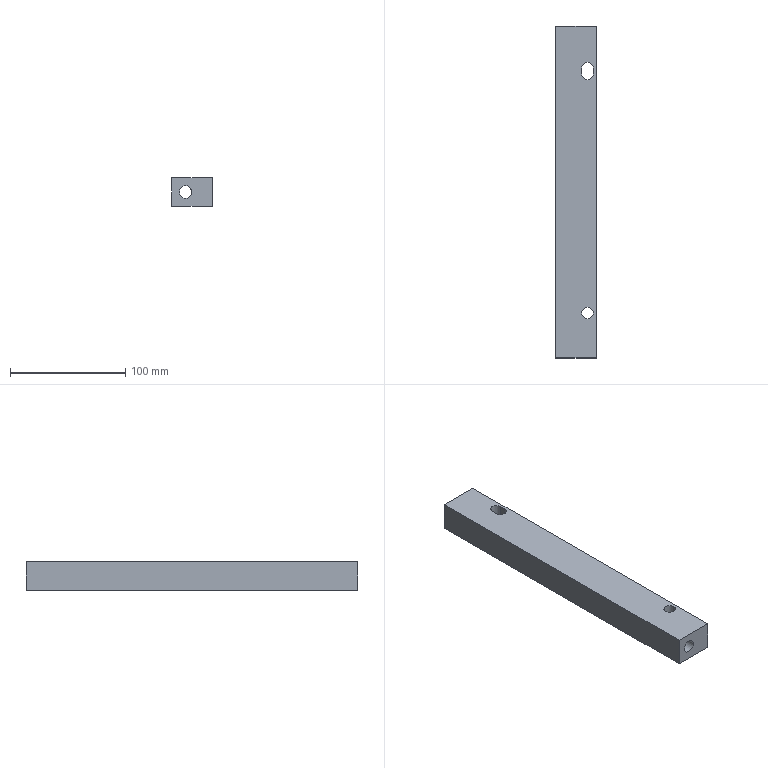Part | NX | features solid 2 | 1 solid | 19 faces | box 35 x 288 x 25 mm | volume 207259 mm3 | cylinder 11 | plane 8 | commonest cylinder face diameters 11 x8 10 x3
STEP:
#1=CARTESIAN_POINT('',(42.5,-250.,340.));
#2=VERTEX_POINT('',#1);
#3=CARTESIAN_POINT('',(47.5,-250.,340.));
#4=DIRECTION('',(0.,0.,-1.));
#5=DIRECTION('',(-1.,0.,0.));
#6=AXIS2_PLACEMENT_3D('',#3,#4,#5);
#7=CIRCLE('',#6,5.);
#8=EDGE_CURVE('',#2,#2,#7,.T.);
#9=ORIENTED_EDGE('',*,*,#8,.T.);
#10=EDGE_LOOP('',(#9));
#11=FACE_BOUND('',#10,.T.);
#12=CARTESIAN_POINT('',(52.5,-37.5,340.));
#13=VERTEX_POINT('',#12);
#14=CARTESIAN_POINT('',(52.5,-42.5,340.));
#15=VERTEX_POINT('',#14);
#16=CARTESIAN_POINT('',(52.5,-145.,340.));
#17=DIRECTION('',(0.,-1.,0.));
#18=VECTOR('',#17,1000.);
#19=LINE('',#16,#18);
#20=EDGE_CURVE('',#13,#15,#19,.T.);
#21=ORIENTED_EDGE('',*,*,#20,.T.);
#22=CARTESIAN_POINT('',(42.5,-42.5,340.));
#23=VERTEX_POINT('',#22);
#24=CARTESIAN_POINT('',(47.5,-42.5,340.));
#25=DIRECTION('',(0.,0.,-1.));
#26=DIRECTION('',(-1.,0.,0.));
#27=AXIS2_PLACEMENT_3D('',#24,#25,#26);
#28=CIRCLE('',#27,5.);
#29=EDGE_CURVE('',#15,#23,#28,.T.);
#30=ORIENTED_EDGE('',*,*,#29,.T.);
#31=CARTESIAN_POINT('',(42.5,-37.5,340.));
#32=VERTEX_POINT('',#31);
#33=CARTESIAN_POINT('',(42.5,-145.,340.));
#34=DIRECTION('',(0.,1.,0.));
#35=VECTOR('',#34,1000.);
#36=LINE('',#33,#35);
#37=EDGE_CURVE('',#23,#32,#36,.T.);
#38=ORIENTED_EDGE('',*,*,#37,.T.);
#39=CARTESIAN_POINT('',(47.5,-37.5,340.));
#40=DIRECTION('',(0.,0.,-1.));
#41=DIRECTION('',(-1.,0.,0.));
#42=AXIS2_PLACEMENT_3D('',#39,#40,#41);
#43=CIRCLE('',#42,5.);
#44=EDGE_CURVE('',#32,#13,#43,.T.);
#45=ORIENTED_EDGE('',*,*,#44,.T.);
#46=EDGE_LOOP('',(#21,#30,#38,#45));
#47=FACE_BOUND('',#46,.T.);
#48=CARTESIAN_POINT('',(20.,-289.,340.));
#49=VERTEX_POINT('',#48);
#50=CARTESIAN_POINT('',(55.,-289.,340.));
#51=VERTEX_POINT('',#50);
#52=CARTESIAN_POINT('',(37.5,-289.,340.));
#53=DIRECTION('',(1.,0.,0.));
#54=VECTOR('',#53,1000.);
#55=LINE('',#52,#54);
#56=EDGE_CURVE('',#49,#51,#55,.T.);
#57=ORIENTED_EDGE('',*,*,#56,.T.);
#58=CARTESIAN_POINT('',(55.,-1.,340.));
#59=VERTEX_POINT('',#58);
#60=CARTESIAN_POINT('',(55.,-145.,340.));
#61=DIRECTION('',(0.,1.,0.));
#62=VECTOR('',#61,1000.);
#63=LINE('',#60,#62);
#64=EDGE_CURVE('',#51,#59,#63,.T.);
#65=ORIENTED_EDGE('',*,*,#64,.T.);
#66=CARTESIAN_POINT('',(20.,-1.,340.));
#67=VERTEX_POINT('',#66);
#68=CARTESIAN_POINT('',(37.5,-1.,340.));
#69=DIRECTION('',(-1.,0.,0.));
#70=VECTOR('',#69,1000.);
#71=LINE('',#68,#70);
#72=EDGE_CURVE('',#59,#67,#71,.T.);
#73=ORIENTED_EDGE('',*,*,#72,.T.);
#74=CARTESIAN_POINT('',(20.,-145.,340.));
#75=DIRECTION('',(0.,-1.,0.));
#76=VECTOR('',#75,1000.);
#77=LINE('',#74,#76);
#78=EDGE_CURVE('',#67,#49,#77,.T.);
#79=ORIENTED_EDGE('',*,*,#78,.T.);
#80=EDGE_LOOP('',(#57,#65,#73,#79));
#81=FACE_BOUND('',#80,.T.);
#82=CARTESIAN_POINT('',(37.5,-145.,340.));
#83=DIRECTION('',(0.,0.,1.));
#84=DIRECTION('',(-1.,0.,0.));
#85=AXIS2_PLACEMENT_3D('',#82,#83,#84);
#86=PLANE('',#85);
#87=ADVANCED_FACE('',(#11,#47,#81),#86,.T.);
#88=CARTESIAN_POINT('',(32.,-289.,322.));
#89=VERTEX_POINT('',#88);
#90=CARTESIAN_POINT('',(32.,-289.,327.5));
#91=DIRECTION('',(0.,1.,0.));
#92=DIRECTION('',(0.,0.,-1.));
#93=AXIS2_PLACEMENT_3D('',#90,#91,#92);
#94=CIRCLE('',#93,5.5);
#95=EDGE_CURVE('',#89,#89,#94,.T.);
#96=ORIENTED_EDGE('',*,*,#95,.T.);
#97=EDGE_LOOP('',(#96));
#98=FACE_BOUND('',#97,.T.);
#99=CARTESIAN_POINT('',(20.,-289.,315.));
#100=VERTEX_POINT('',#99);
#101=CARTESIAN_POINT('',(20.,-289.,315.));
#102=DIRECTION('',(0.,0.,1.));
#103=VECTOR('',#102,1000.);
#104=LINE('',#101,#103);
#105=EDGE_CURVE('',#100,#49,#104,.T.);
#106=ORIENTED_EDGE('',*,*,#105,.F.);
#107=CARTESIAN_POINT('',(55.,-289.,315.));
#108=VERTEX_POINT('',#107);
#109=CARTESIAN_POINT('',(37.5,-289.,315.));
#110=DIRECTION('',(-1.,0.,0.));
#111=VECTOR('',#110,1000.);
#112=LINE('',#109,#111);
#113=EDGE_CURVE('',#108,#100,#112,.T.);
#114=ORIENTED_EDGE('',*,*,#113,.F.);
#115=CARTESIAN_POINT('',(55.,-289.,315.));
#116=DIRECTION('',(0.,0.,1.));
#117=VECTOR('',#116,1000.);
#118=LINE('',#115,#117);
#119=EDGE_CURVE('',#108,#51,#118,.T.);
#120=ORIENTED_EDGE('',*,*,#119,.T.);
#121=ORIENTED_EDGE('',*,*,#56,.F.);
#122=EDGE_LOOP('',(#106,#114,#120,#121));
#123=FACE_BOUND('',#122,.T.);
#124=CARTESIAN_POINT('',(37.5,-289.,315.));
#125=DIRECTION('',(0.,-1.,0.));
#126=DIRECTION('',(0.,0.,-1.));
#127=AXIS2_PLACEMENT_3D('',#124,#125,#126);
#128=PLANE('',#127);
#129=ADVANCED_FACE('',(#98,#123),#128,.T.);
#130=CARTESIAN_POINT('',(55.,-271.,322.));
#131=VERTEX_POINT('',#130);
#132=CARTESIAN_POINT('',(55.,-271.,327.5));
#133=DIRECTION('',(1.,0.,0.));
#134=DIRECTION('',(0.,0.,-1.));
#135=AXIS2_PLACEMENT_3D('',#132,#133,#134);
#136=CIRCLE('',#135,5.5);
#137=EDGE_CURVE('',#131,#131,#136,.T.);
#138=ORIENTED_EDGE('',*,*,#137,.F.);
#139=EDGE_LOOP('',(#138));
#140=FACE_BOUND('',#139,.T.);
#141=CARTESIAN_POINT('',(55.,-229.,322.));
#142=VERTEX_POINT('',#141);
#143=CARTESIAN_POINT('',(55.,-229.,327.5));
#144=DIRECTION('',(1.,0.,0.));
#145=DIRECTION('',(0.,0.,-1.));
#146=AXIS2_PLACEMENT_3D('',#143,#144,#145);
#147=CIRCLE('',#146,5.5);
#148=EDGE_CURVE('',#142,#142,#147,.T.);
#149=ORIENTED_EDGE('',*,*,#148,.F.);
#150=EDGE_LOOP('',(#149));
#151=FACE_BOUND('',#150,.T.);
#152=CARTESIAN_POINT('',(55.,-187.,322.));
#153=VERTEX_POINT('',#152);
#154=CARTESIAN_POINT('',(55.,-187.,327.5));
#155=DIRECTION('',(1.,0.,0.));
#156=DIRECTION('',(0.,0.,-1.));
#157=AXIS2_PLACEMENT_3D('',#154,#155,#156);
#158=CIRCLE('',#157,5.5);
#159=EDGE_CURVE('',#153,#153,#158,.T.);
#160=ORIENTED_EDGE('',*,*,#159,.F.);
#161=EDGE_LOOP('',(#160));
#162=FACE_BOUND('',#161,.T.);
#163=CARTESIAN_POINT('',(55.,-145.,322.));
#164=VERTEX_POINT('',#163);
#165=CARTESIAN_POINT('',(55.,-145.,327.5));
#166=DIRECTION('',(1.,0.,0.));
#167=DIRECTION('',(0.,0.,-1.));
#168=AXIS2_PLACEMENT_3D('',#165,#166,#167);
#169=CIRCLE('',#168,5.5);
#170=EDGE_CURVE('',#164,#164,#169,.T.);
#171=ORIENTED_EDGE('',*,*,#170,.F.);
#172=EDGE_LOOP('',(#171));
#173=FACE_BOUND('',#172,.T.);
#174=CARTESIAN_POINT('',(55.,-103.,322.));
#175=VERTEX_POINT('',#174);
#176=CARTESIAN_POINT('',(55.,-103.,327.5));
#177=DIRECTION('',(1.,0.,0.));
#178=DIRECTION('',(0.,0.,-1.));
#179=AXIS2_PLACEMENT_3D('',#176,#177,#178);
#180=CIRCLE('',#179,5.5);
#181=EDGE_CURVE('',#175,#175,#180,.T.);
#182=ORIENTED_EDGE('',*,*,#181,.F.);
#183=EDGE_LOOP('',(#182));
#184=FACE_BOUND('',#183,.T.);
#185=CARTESIAN_POINT('',(55.,-61.,322.));
#186=VERTEX_POINT('',#185);
#187=CARTESIAN_POINT('',(55.,-61.,327.5));
#188=DIRECTION('',(1.,0.,0.));
#189=DIRECTION('',(0.,0.,-1.));
#190=AXIS2_PLACEMENT_3D('',#187,#188,#189);
#191=CIRCLE('',#190,5.5);
#192=EDGE_CURVE('',#186,#186,#191,.T.);
#193=ORIENTED_EDGE('',*,*,#192,.F.);
#194=EDGE_LOOP('',(#193));
#195=FACE_BOUND('',#194,.T.);
#196=CARTESIAN_POINT('',(55.,-19.,322.));
#197=VERTEX_POINT('',#196);
#198=CARTESIAN_POINT('',(55.,-19.,327.5));
#199=DIRECTION('',(1.,0.,0.));
#200=DIRECTION('',(0.,0.,-1.));
#201=AXIS2_PLACEMENT_3D('',#198,#199,#200);
#202=CIRCLE('',#201,5.5);
#203=EDGE_CURVE('',#197,#197,#202,.T.);
#204=ORIENTED_EDGE('',*,*,#203,.F.);
#205=EDGE_LOOP('',(#204));
#206=FACE_BOUND('',#205,.T.);
#207=ORIENTED_EDGE('',*,*,#119,.F.);
#208=CARTESIAN_POINT('',(55.,-1.,315.));
#209=VERTEX_POINT('',#208);
#210=CARTESIAN_POINT('',(55.,-145.,315.));
#211=DIRECTION('',(0.,-1.,0.));
#212=VECTOR('',#211,1000.);
#213=LINE('',#210,#212);
#214=EDGE_CURVE('',#209,#108,#213,.T.);
#215=ORIENTED_EDGE('',*,*,#214,.F.);
#216=CARTESIAN_POINT('',(55.,-1.,315.));
#217=DIRECTION('',(0.,0.,1.));
#218=VECTOR('',#217,1000.);
#219=LINE('',#216,#218);
#220=EDGE_CURVE('',#209,#59,#219,.T.);
#221=ORIENTED_EDGE('',*,*,#220,.T.);
#222=ORIENTED_EDGE('',*,*,#64,.F.);
#223=EDGE_LOOP('',(#207,#215,#221,#222));
#224=FACE_BOUND('',#223,.T.);
#225=CARTESIAN_POINT('',(55.,-145.,315.));
#226=DIRECTION('',(1.,0.,0.));
#227=DIRECTION('',(0.,0.,1.));
#228=AXIS2_PLACEMENT_3D('',#225,#226,#227);
#229=PLANE('',#228);
#230=ADVANCED_FACE('',(#140,#151,#162,#173,#184,#195,#206,#224),#229,.T.);
#231=CARTESIAN_POINT('',(32.,-1.,322.));
#232=VERTEX_POINT('',#231);
#233=CARTESIAN_POINT('',(32.,-1.,327.5));
#234=DIRECTION('',(0.,1.,0.));
#235=DIRECTION('',(0.,0.,-1.));
#236=AXIS2_PLACEMENT_3D('',#233,#234,#235);
#237=CIRCLE('',#236,5.5);
#238=EDGE_CURVE('',#232,#232,#237,.T.);
#239=ORIENTED_EDGE('',*,*,#238,.F.);
#240=EDGE_LOOP('',(#239));
#241=FACE_BOUND('',#240,.T.);
#242=ORIENTED_EDGE('',*,*,#220,.F.);
#243=CARTESIAN_POINT('',(20.,-1.,315.));
#244=VERTEX_POINT('',#243);
#245=CARTESIAN_POINT('',(37.5,-1.,315.));
#246=DIRECTION('',(1.,0.,0.));
#247=VECTOR('',#246,1000.);
#248=LINE('',#245,#247);
#249=EDGE_CURVE('',#244,#209,#248,.T.);
#250=ORIENTED_EDGE('',*,*,#249,.F.);
#251=CARTESIAN_POINT('',(20.,-1.,315.));
#252=DIRECTION('',(0.,0.,1.));
#253=VECTOR('',#252,1000.);
#254=LINE('',#251,#253);
#255=EDGE_CURVE('',#244,#67,#254,.T.);
#256=ORIENTED_EDGE('',*,*,#255,.T.);
#257=ORIENTED_EDGE('',*,*,#72,.F.);
#258=EDGE_LOOP('',(#242,#250,#256,#257));
#259=FACE_BOUND('',#258,.T.);
#260=CARTESIAN_POINT('',(37.5,-1.,315.));
#261=DIRECTION('',(0.,1.,0.));
#262=DIRECTION('',(0.,0.,1.));
#263=AXIS2_PLACEMENT_3D('',#260,#261,#262);
#264=PLANE('',#263);
#265=ADVANCED_FACE('',(#241,#259),#264,.T.);
#266=CARTESIAN_POINT('',(42.5,-250.,315.));
#267=VERTEX_POINT('',#266);
#268=CARTESIAN_POINT('',(47.5,-250.,315.));
#269=DIRECTION('',(0.,0.,-1.));
#270=DIRECTION('',(-1.,0.,0.));
#271=AXIS2_PLACEMENT_3D('',#268,#269,#270);
#272=CIRCLE('',#271,5.);
#273=EDGE_CURVE('',#267,#267,#272,.T.);
#274=ORIENTED_EDGE('',*,*,#273,.F.);
#275=EDGE_LOOP('',(#274));
#276=FACE_BOUND('',#275,.T.);
#277=CARTESIAN_POINT('',(52.5,-37.5,315.));
#278=VERTEX_POINT('',#277);
#279=CARTESIAN_POINT('',(52.5,-42.5,315.));
#280=VERTEX_POINT('',#279);
#281=CARTESIAN_POINT('',(52.5,-40.,315.));
#282=DIRECTION('',(0.,-1.,0.));
#283=VECTOR('',#282,1000.);
#284=LINE('',#281,#283);
#285=EDGE_CURVE('',#278,#280,#284,.T.);
#286=ORIENTED_EDGE('',*,*,#285,.F.);
#287=CARTESIAN_POINT('',(42.5,-37.5,315.));
#288=VERTEX_POINT('',#287);
#289=CARTESIAN_POINT('',(47.5,-37.5,315.));
#290=DIRECTION('',(0.,0.,1.));
#291=DIRECTION('',(1.,0.,0.));
#292=AXIS2_PLACEMENT_3D('',#289,#290,#291);
#293=CIRCLE('',#292,5.);
#294=EDGE_CURVE('',#278,#288,#293,.T.);
#295=ORIENTED_EDGE('',*,*,#294,.T.);
#296=CARTESIAN_POINT('',(42.5,-42.5,315.));
#297=VERTEX_POINT('',#296);
#298=CARTESIAN_POINT('',(42.5,-40.,315.));
#299=DIRECTION('',(0.,-1.,0.));
#300=VECTOR('',#299,1000.);
#301=LINE('',#298,#300);
#302=EDGE_CURVE('',#288,#297,#301,.T.);
#303=ORIENTED_EDGE('',*,*,#302,.T.);
#304=CARTESIAN_POINT('',(47.5,-42.5,315.));
#305=DIRECTION('',(0.,0.,1.));
#306=DIRECTION('',(1.,0.,0.));
#307=AXIS2_PLACEMENT_3D('',#304,#305,#306);
#308=CIRCLE('',#307,5.);
#309=EDGE_CURVE('',#297,#280,#308,.T.);
#310=ORIENTED_EDGE('',*,*,#309,.T.);
#311=EDGE_LOOP('',(#286,#295,#303,#310));
#312=FACE_BOUND('',#311,.T.);
#313=CARTESIAN_POINT('',(20.,-145.,315.));
#314=DIRECTION('',(0.,1.,0.));
#315=VECTOR('',#314,1000.);
#316=LINE('',#313,#315);
#317=EDGE_CURVE('',#100,#244,#316,.T.);
#318=ORIENTED_EDGE('',*,*,#317,.T.);
#319=ORIENTED_EDGE('',*,*,#249,.T.);
#320=ORIENTED_EDGE('',*,*,#214,.T.);
#321=ORIENTED_EDGE('',*,*,#113,.T.);
#322=EDGE_LOOP('',(#318,#319,#320,#321));
#323=FACE_BOUND('',#322,.T.);
#324=CARTESIAN_POINT('',(37.5,-145.,315.));
#325=DIRECTION('',(0.,0.,-1.));
#326=DIRECTION('',(1.,0.,0.));
#327=AXIS2_PLACEMENT_3D('',#324,#325,#326);
#328=PLANE('',#327);
#329=ADVANCED_FACE('',(#276,#312,#323),#328,.T.);
#330=ORIENTED_EDGE('',*,*,#317,.F.);
#331=ORIENTED_EDGE('',*,*,#105,.T.);
#332=ORIENTED_EDGE('',*,*,#78,.F.);
#333=ORIENTED_EDGE('',*,*,#255,.F.);
#334=EDGE_LOOP('',(#330,#331,#332,#333));
#335=FACE_BOUND('',#334,.T.);
#336=CARTESIAN_POINT('',(20.,-145.,315.));
#337=DIRECTION('',(-1.,0.,0.));
#338=DIRECTION('',(0.,0.,-1.));
#339=AXIS2_PLACEMENT_3D('',#336,#337,#338);
#340=PLANE('',#339);
#341=ADVANCED_FACE('',(#335),#340,.T.);
#342=CARTESIAN_POINT('',(32.,-271.,333.));
#343=VERTEX_POINT('',#342);
#344=CARTESIAN_POINT('',(32.,-271.,322.));
#345=VERTEX_POINT('',#344);
#346=CARTESIAN_POINT('',(32.,-271.,327.5));
#347=DIRECTION('',(-0.7071,0.7071,0.));
#348=DIRECTION('',(-0.7071,-0.7071,0.));
#349=AXIS2_PLACEMENT_3D('',#346,#347,#348);
#350=ELLIPSE('',#349,7.778,5.5);
#351=EDGE_CURVE('',#343,#345,#350,.T.);
#352=ORIENTED_EDGE('',*,*,#351,.F.);
#353=CARTESIAN_POINT('',(32.,-271.,327.5));
#354=DIRECTION('',(0.7071,0.7071,0.));
#355=DIRECTION('',(0.7071,-0.7071,0.));
#356=AXIS2_PLACEMENT_3D('',#353,#354,#355);
#357=ELLIPSE('',#356,7.778,5.5);
#358=EDGE_CURVE('',#345,#343,#357,.F.);
#359=ORIENTED_EDGE('',*,*,#358,.F.);
#360=EDGE_LOOP('',(#352,#359));
#361=FACE_BOUND('',#360,.T.);
#362=CARTESIAN_POINT('',(32.,-229.,333.));
#363=VERTEX_POINT('',#362);
#364=CARTESIAN_POINT('',(32.,-229.,322.));
#365=VERTEX_POINT('',#364);
#366=CARTESIAN_POINT('',(32.,-229.,327.5));
#367=DIRECTION('',(-0.7071,0.7071,0.));
#368=DIRECTION('',(-0.7071,-0.7071,0.));
#369=AXIS2_PLACEMENT_3D('',#366,#367,#368);
#370=ELLIPSE('',#369,7.778,5.5);
#371=EDGE_CURVE('',#363,#365,#370,.T.);
#372=ORIENTED_EDGE('',*,*,#371,.F.);
#373=CARTESIAN_POINT('',(32.,-229.,327.5));
#374=DIRECTION('',(0.7071,0.7071,0.));
#375=DIRECTION('',(0.7071,-0.7071,0.));
#376=AXIS2_PLACEMENT_3D('',#373,#374,#375);
#377=ELLIPSE('',#376,7.778,5.5);
#378=EDGE_CURVE('',#365,#363,#377,.F.);
#379=ORIENTED_EDGE('',*,*,#378,.F.);
#380=EDGE_LOOP('',(#372,#379));
#381=FACE_BOUND('',#380,.T.);
#382=CARTESIAN_POINT('',(32.,-187.,333.));
#383=VERTEX_POINT('',#382);
#384=CARTESIAN_POINT('',(32.,-187.,322.));
#385=VERTEX_POINT('',#384);
#386=CARTESIAN_POINT('',(32.,-187.,327.5));
#387=DIRECTION('',(-0.7071,0.7071,0.));
#388=DIRECTION('',(-0.7071,-0.7071,0.));
#389=AXIS2_PLACEMENT_3D('',#386,#387,#388);
#390=ELLIPSE('',#389,7.778,5.5);
#391=EDGE_CURVE('',#383,#385,#390,.T.);
#392=ORIENTED_EDGE('',*,*,#391,.F.);
#393=CARTESIAN_POINT('',(32.,-187.,327.5));
#394=DIRECTION('',(0.7071,0.7071,0.));
#395=DIRECTION('',(0.7071,-0.7071,0.));
#396=AXIS2_PLACEMENT_3D('',#393,#394,#395);
#397=ELLIPSE('',#396,7.778,5.5);
#398=EDGE_CURVE('',#385,#383,#397,.F.);
#399=ORIENTED_EDGE('',*,*,#398,.F.);
#400=EDGE_LOOP('',(#392,#399));
#401=FACE_BOUND('',#400,.T.);
#402=CARTESIAN_POINT('',(32.,-145.,333.));
#403=VERTEX_POINT('',#402);
#404=CARTESIAN_POINT('',(32.,-145.,322.));
#405=VERTEX_POINT('',#404);
#406=CARTESIAN_POINT('',(32.,-145.,327.5));
#407=DIRECTION('',(-0.7071,0.7071,0.));
#408=DIRECTION('',(-0.7071,-0.7071,0.));
#409=AXIS2_PLACEMENT_3D('',#406,#407,#408);
#410=ELLIPSE('',#409,7.778,5.5);
#411=EDGE_CURVE('',#403,#405,#410,.T.);
#412=ORIENTED_EDGE('',*,*,#411,.F.);
#413=CARTESIAN_POINT('',(32.,-145.,327.5));
#414=DIRECTION('',(0.7071,0.7071,0.));
#415=DIRECTION('',(0.7071,-0.7071,0.));
#416=AXIS2_PLACEMENT_3D('',#413,#414,#415);
#417=ELLIPSE('',#416,7.778,5.5);
#418=EDGE_CURVE('',#405,#403,#417,.F.);
#419=ORIENTED_EDGE('',*,*,#418,.F.);
#420=EDGE_LOOP('',(#412,#419));
#421=FACE_BOUND('',#420,.T.);
#422=CARTESIAN_POINT('',(32.,-103.,333.));
#423=VERTEX_POINT('',#422);
#424=CARTESIAN_POINT('',(32.,-103.,322.));
#425=VERTEX_POINT('',#424);
#426=CARTESIAN_POINT('',(32.,-103.,327.5));
#427=DIRECTION('',(-0.7071,0.7071,0.));
#428=DIRECTION('',(-0.7071,-0.7071,0.));
#429=AXIS2_PLACEMENT_3D('',#426,#427,#428);
#430=ELLIPSE('',#429,7.778,5.5);
#431=EDGE_CURVE('',#423,#425,#430,.T.);
#432=ORIENTED_EDGE('',*,*,#431,.F.);
#433=CARTESIAN_POINT('',(32.,-103.,327.5));
#434=DIRECTION('',(0.7071,0.7071,0.));
#435=DIRECTION('',(0.7071,-0.7071,0.));
#436=AXIS2_PLACEMENT_3D('',#433,#434,#435);
#437=ELLIPSE('',#436,7.778,5.5);
#438=EDGE_CURVE('',#425,#423,#437,.F.);
#439=ORIENTED_EDGE('',*,*,#438,.F.);
#440=EDGE_LOOP('',(#432,#439));
#441=FACE_BOUND('',#440,.T.);
#442=CARTESIAN_POINT('',(32.,-61.,333.));
#443=VERTEX_POINT('',#442);
#444=CARTESIAN_POINT('',(32.,-61.,322.));
#445=VERTEX_POINT('',#444);
#446=CARTESIAN_POINT('',(32.,-61.,327.5));
#447=DIRECTION('',(-0.7071,0.7071,0.));
#448=DIRECTION('',(-0.7071,-0.7071,0.));
#449=AXIS2_PLACEMENT_3D('',#446,#447,#448);
#450=ELLIPSE('',#449,7.778,5.5);
#451=EDGE_CURVE('',#443,#445,#450,.T.);
#452=ORIENTED_EDGE('',*,*,#451,.F.);
#453=CARTESIAN_POINT('',(32.,-61.,327.5));
#454=DIRECTION('',(0.7071,0.7071,0.));
#455=DIRECTION('',(0.7071,-0.7071,0.));
#456=AXIS2_PLACEMENT_3D('',#453,#454,#455);
#457=ELLIPSE('',#456,7.778,5.5);
#458=EDGE_CURVE('',#445,#443,#457,.F.);
#459=ORIENTED_EDGE('',*,*,#458,.F.);
#460=EDGE_LOOP('',(#452,#459));
#461=FACE_BOUND('',#460,.T.);
#462=CARTESIAN_POINT('',(32.,-19.,333.));
#463=VERTEX_POINT('',#462);
#464=CARTESIAN_POINT('',(32.,-19.,322.));
#465=VERTEX_POINT('',#464);
#466=CARTESIAN_POINT('',(32.,-19.,327.5));
#467=DIRECTION('',(-0.7071,0.7071,0.));
#468=DIRECTION('',(-0.7071,-0.7071,0.));
#469=AXIS2_PLACEMENT_3D('',#466,#467,#468);
#470=ELLIPSE('',#469,7.778,5.5);
#471=EDGE_CURVE('',#463,#465,#470,.T.);
#472=ORIENTED_EDGE('',*,*,#471,.F.);
#473=CARTESIAN_POINT('',(32.,-19.,327.5));
#474=DIRECTION('',(0.7071,0.7071,0.));
#475=DIRECTION('',(0.7071,-0.7071,0.));
#476=AXIS2_PLACEMENT_3D('',#473,#474,#475);
#477=ELLIPSE('',#476,7.778,5.5);
#478=EDGE_CURVE('',#465,#463,#477,.F.);
#479=ORIENTED_EDGE('',*,*,#478,.F.);
#480=EDGE_LOOP('',(#472,#479));
#481=FACE_BOUND('',#480,.T.);
#482=ORIENTED_EDGE('',*,*,#95,.F.);
#483=EDGE_LOOP('',(#482));
#484=FACE_BOUND('',#483,.T.);
#485=ORIENTED_EDGE('',*,*,#238,.T.);
#486=EDGE_LOOP('',(#485));
#487=FACE_BOUND('',#486,.T.);
#488=CARTESIAN_POINT('',(32.,-1.,327.5));
#489=DIRECTION('',(0.,-1.,0.));
#490=DIRECTION('',(0.,0.,-1.));
#491=AXIS2_PLACEMENT_3D('',#488,#489,#490);
#492=CYLINDRICAL_SURFACE('',#491,5.5);
#493=ADVANCED_FACE('',(#361,#381,#401,#421,#441,#461,#481,#484,#487),#492,.F.);
#494=ORIENTED_EDGE('',*,*,#203,.T.);
#495=EDGE_LOOP('',(#494));
#496=FACE_BOUND('',#495,.T.);
#497=ORIENTED_EDGE('',*,*,#471,.T.);
#498=ORIENTED_EDGE('',*,*,#478,.T.);
#499=EDGE_LOOP('',(#497,#498));
#500=FACE_BOUND('',#499,.T.);
#501=CARTESIAN_POINT('',(55.,-19.,327.5));
#502=DIRECTION('',(-1.,0.,0.));
#503=DIRECTION('',(0.,0.,-1.));
#504=AXIS2_PLACEMENT_3D('',#501,#502,#503);
#505=CYLINDRICAL_SURFACE('',#504,5.5);
#506=ADVANCED_FACE('',(#496,#500),#505,.F.);
#507=ORIENTED_EDGE('',*,*,#192,.T.);
#508=EDGE_LOOP('',(#507));
#509=FACE_BOUND('',#508,.T.);
#510=ORIENTED_EDGE('',*,*,#451,.T.);
#511=ORIENTED_EDGE('',*,*,#458,.T.);
#512=EDGE_LOOP('',(#510,#511));
#513=FACE_BOUND('',#512,.T.);
#514=CARTESIAN_POINT('',(55.,-61.,327.5));
#515=DIRECTION('',(-1.,0.,0.));
#516=DIRECTION('',(0.,0.,-1.));
#517=AXIS2_PLACEMENT_3D('',#514,#515,#516);
#518=CYLINDRICAL_SURFACE('',#517,5.5);
#519=ADVANCED_FACE('',(#509,#513),#518,.F.);
#520=ORIENTED_EDGE('',*,*,#181,.T.);
#521=EDGE_LOOP('',(#520));
#522=FACE_BOUND('',#521,.T.);
#523=ORIENTED_EDGE('',*,*,#431,.T.);
#524=ORIENTED_EDGE('',*,*,#438,.T.);
#525=EDGE_LOOP('',(#523,#524));
#526=FACE_BOUND('',#525,.T.);
#527=CARTESIAN_POINT('',(55.,-103.,327.5));
#528=DIRECTION('',(-1.,0.,0.));
#529=DIRECTION('',(0.,0.,-1.));
#530=AXIS2_PLACEMENT_3D('',#527,#528,#529);
#531=CYLINDRICAL_SURFACE('',#530,5.5);
#532=ADVANCED_FACE('',(#522,#526),#531,.F.);
#533=ORIENTED_EDGE('',*,*,#170,.T.);
#534=EDGE_LOOP('',(#533));
#535=FACE_BOUND('',#534,.T.);
#536=ORIENTED_EDGE('',*,*,#411,.T.);
#537=ORIENTED_EDGE('',*,*,#418,.T.);
#538=EDGE_LOOP('',(#536,#537));
#539=FACE_BOUND('',#538,.T.);
#540=CARTESIAN_POINT('',(55.,-145.,327.5));
#541=DIRECTION('',(-1.,0.,0.));
#542=DIRECTION('',(0.,0.,-1.));
#543=AXIS2_PLACEMENT_3D('',#540,#541,#542);
#544=CYLINDRICAL_SURFACE('',#543,5.5);
#545=ADVANCED_FACE('',(#535,#539),#544,.F.);
#546=ORIENTED_EDGE('',*,*,#159,.T.);
#547=EDGE_LOOP('',(#546));
#548=FACE_BOUND('',#547,.T.);
#549=ORIENTED_EDGE('',*,*,#391,.T.);
#550=ORIENTED_EDGE('',*,*,#398,.T.);
#551=EDGE_LOOP('',(#549,#550));
#552=FACE_BOUND('',#551,.T.);
#553=CARTESIAN_POINT('',(55.,-187.,327.5));
#554=DIRECTION('',(-1.,0.,0.));
#555=DIRECTION('',(0.,0.,-1.));
#556=AXIS2_PLACEMENT_3D('',#553,#554,#555);
#557=CYLINDRICAL_SURFACE('',#556,5.5);
#558=ADVANCED_FACE('',(#548,#552),#557,.F.);
#559=ORIENTED_EDGE('',*,*,#148,.T.);
#560=EDGE_LOOP('',(#559));
#561=FACE_BOUND('',#560,.T.);
#562=ORIENTED_EDGE('',*,*,#371,.T.);
#563=ORIENTED_EDGE('',*,*,#378,.T.);
#564=EDGE_LOOP('',(#562,#563));
#565=FACE_BOUND('',#564,.T.);
#566=CARTESIAN_POINT('',(55.,-229.,327.5));
#567=DIRECTION('',(-1.,0.,0.));
#568=DIRECTION('',(0.,0.,-1.));
#569=AXIS2_PLACEMENT_3D('',#566,#567,#568);
#570=CYLINDRICAL_SURFACE('',#569,5.5);
#571=ADVANCED_FACE('',(#561,#565),#570,.F.);
#572=ORIENTED_EDGE('',*,*,#137,.T.);
#573=EDGE_LOOP('',(#572));
#574=FACE_BOUND('',#573,.T.);
#575=ORIENTED_EDGE('',*,*,#351,.T.);
#576=ORIENTED_EDGE('',*,*,#358,.T.);
#577=EDGE_LOOP('',(#575,#576));
#578=FACE_BOUND('',#577,.T.);
#579=CARTESIAN_POINT('',(55.,-271.,327.5));
#580=DIRECTION('',(-1.,0.,0.));
#581=DIRECTION('',(0.,0.,-1.));
#582=AXIS2_PLACEMENT_3D('',#579,#580,#581);
#583=CYLINDRICAL_SURFACE('',#582,5.5);
#584=ADVANCED_FACE('',(#574,#578),#583,.F.);
#585=ORIENTED_EDGE('',*,*,#20,.F.);
#586=CARTESIAN_POINT('',(52.5,-37.5,315.));
#587=DIRECTION('',(0.,0.,-1.));
#588=VECTOR('',#587,1000.);
#589=LINE('',#586,#588);
#590=EDGE_CURVE('',#13,#278,#589,.T.);
#591=ORIENTED_EDGE('',*,*,#590,.T.);
#592=ORIENTED_EDGE('',*,*,#285,.T.);
#593=CARTESIAN_POINT('',(52.5,-42.5,315.));
#594=DIRECTION('',(0.,0.,-1.));
#595=VECTOR('',#594,1000.);
#596=LINE('',#593,#595);
#597=EDGE_CURVE('',#15,#280,#596,.T.);
#598=ORIENTED_EDGE('',*,*,#597,.F.);
#599=EDGE_LOOP('',(#585,#591,#592,#598));
#600=FACE_BOUND('',#599,.T.);
#601=CARTESIAN_POINT('',(52.5,-40.,315.));
#602=DIRECTION('',(1.,0.,0.));
#603=DIRECTION('',(0.,0.,1.));
#604=AXIS2_PLACEMENT_3D('',#601,#602,#603);
#605=PLANE('',#604);
#606=ADVANCED_FACE('',(#600),#605,.F.);
#607=ORIENTED_EDGE('',*,*,#44,.F.);
#608=CARTESIAN_POINT('',(42.5,-37.5,315.));
#609=DIRECTION('',(0.,0.,-1.));
#610=VECTOR('',#609,1000.);
#611=LINE('',#608,#610);
#612=EDGE_CURVE('',#32,#288,#611,.T.);
#613=ORIENTED_EDGE('',*,*,#612,.T.);
#614=ORIENTED_EDGE('',*,*,#294,.F.);
#615=ORIENTED_EDGE('',*,*,#590,.F.);
#616=EDGE_LOOP('',(#607,#613,#614,#615));
#617=FACE_BOUND('',#616,.T.);
#618=CARTESIAN_POINT('',(47.5,-37.5,315.));
#619=DIRECTION('',(0.,0.,-1.));
#620=DIRECTION('',(1.,0.,0.));
#621=AXIS2_PLACEMENT_3D('',#618,#619,#620);
#622=CYLINDRICAL_SURFACE('',#621,5.);
#623=ADVANCED_FACE('',(#617),#622,.F.);
#624=ORIENTED_EDGE('',*,*,#37,.F.);
#625=CARTESIAN_POINT('',(42.5,-42.5,315.));
#626=DIRECTION('',(0.,0.,-1.));
#627=VECTOR('',#626,1000.);
#628=LINE('',#625,#627);
#629=EDGE_CURVE('',#23,#297,#628,.T.);
#630=ORIENTED_EDGE('',*,*,#629,.T.);
#631=ORIENTED_EDGE('',*,*,#302,.F.);
#632=ORIENTED_EDGE('',*,*,#612,.F.);
#633=EDGE_LOOP('',(#624,#630,#631,#632));
#634=FACE_BOUND('',#633,.T.);
#635=CARTESIAN_POINT('',(42.5,-40.,315.));
#636=DIRECTION('',(-1.,0.,0.));
#637=DIRECTION('',(0.,0.,-1.));
#638=AXIS2_PLACEMENT_3D('',#635,#636,#637);
#639=PLANE('',#638);
#640=ADVANCED_FACE('',(#634),#639,.F.);
#641=ORIENTED_EDGE('',*,*,#29,.F.);
#642=ORIENTED_EDGE('',*,*,#597,.T.);
#643=ORIENTED_EDGE('',*,*,#309,.F.);
#644=ORIENTED_EDGE('',*,*,#629,.F.);
#645=EDGE_LOOP('',(#641,#642,#643,#644));
#646=FACE_BOUND('',#645,.T.);
#647=CARTESIAN_POINT('',(47.5,-42.5,315.));
#648=DIRECTION('',(0.,0.,-1.));
#649=DIRECTION('',(1.,0.,0.));
#650=AXIS2_PLACEMENT_3D('',#647,#648,#649);
#651=CYLINDRICAL_SURFACE('',#650,5.);
#652=ADVANCED_FACE('',(#646),#651,.F.);
#653=ORIENTED_EDGE('',*,*,#8,.F.);
#654=EDGE_LOOP('',(#653));
#655=FACE_BOUND('',#654,.T.);
#656=ORIENTED_EDGE('',*,*,#273,.T.);
#657=EDGE_LOOP('',(#656));
#658=FACE_BOUND('',#657,.T.);
#659=CARTESIAN_POINT('',(47.5,-250.,315.));
#660=DIRECTION('',(0.,0.,1.));
#661=DIRECTION('',(-1.,0.,0.));
#662=AXIS2_PLACEMENT_3D('',#659,#660,#661);
#663=CYLINDRICAL_SURFACE('',#662,5.);
#664=ADVANCED_FACE('',(#655,#658),#663,.F.);
#665=CLOSED_SHELL('',(#87,#129,#230,#265,#329,#341,#493,#506,#519,#532,#545,#558,#571,#584,#606,#623,#640,#652,#664));
#666=MANIFOLD_SOLID_BREP('',#665);
#667=(LENGTH_UNIT()NAMED_UNIT(*)SI_UNIT(.MILLI.,.METRE.));
#668=UNCERTAINTY_MEASURE_WITH_UNIT(LENGTH_MEASURE(0.00001),#667,'','');
#669=(NAMED_UNIT(*)PLANE_ANGLE_UNIT()SI_UNIT($,.RADIAN.));
#670=(NAMED_UNIT(*)SI_UNIT($,.STERADIAN.)SOLID_ANGLE_UNIT());
#671=(GEOMETRIC_REPRESENTATION_CONTEXT(3)GLOBAL_UNCERTAINTY_ASSIGNED_CONTEXT((#668))GLOBAL_UNIT_ASSIGNED_CONTEXT((#667,#669,#670))REPRESENTATION_CONTEXT('',''));
#672=ADVANCED_BREP_SHAPE_REPRESENTATION('',(#666),#671);